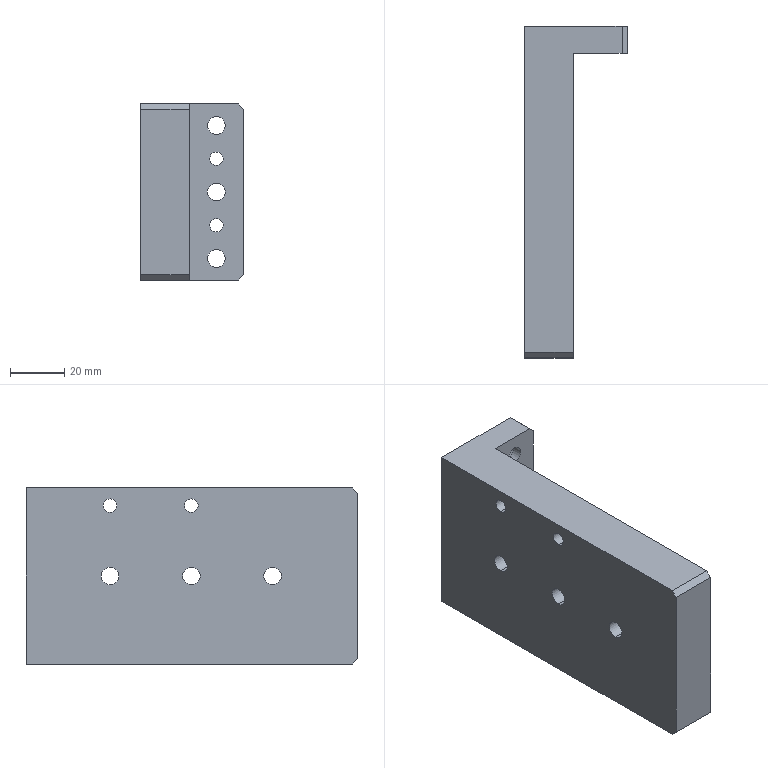Part | SolidWorks | features HoleWzd 4, Cut 2, ICE 2, MoveFace 2, Chamfer 1, Extrusion 1, LibraryFeature 1 | 1 solid | 50 faces | box 38 x 122.5 x 65 mm | volume 149829 mm3 | cylinder 32 | plane 18 | commonest cylinder face diameters 11 x12 5 x8 6.5 x6 6.6 x6
STEP:
#1=CARTESIAN_POINT('',(-8.,31.5,60.75));
#2=VERTEX_POINT('',#1);
#3=CARTESIAN_POINT('',(-8.,31.5,54.25));
#4=VERTEX_POINT('',#3);
#5=CARTESIAN_POINT('',(-8.,31.5,57.5));
#6=DIRECTION('',(1.,0.,0.));
#7=DIRECTION('',(0.,0.,-1.));
#8=AXIS2_PLACEMENT_3D('',#5,#6,#7);
#9=CIRCLE('',#8,3.25);
#10=EDGE_CURVE('',#2,#4,#9,.T.);
#11=ORIENTED_EDGE('',*,*,#10,.F.);
#12=CARTESIAN_POINT('',(3.,31.5,60.75));
#13=VERTEX_POINT('',#12);
#14=CARTESIAN_POINT('',(10.,31.5,60.75));
#15=DIRECTION('',(1.,0.,0.));
#16=VECTOR('',#15,1000.);
#17=LINE('',#14,#16);
#18=EDGE_CURVE('',#2,#13,#17,.T.);
#19=ORIENTED_EDGE('',*,*,#18,.T.);
#20=CARTESIAN_POINT('',(3.,31.5,54.25));
#21=VERTEX_POINT('',#20);
#22=CARTESIAN_POINT('',(3.,31.5,57.5));
#23=DIRECTION('',(1.,0.,0.));
#24=DIRECTION('',(0.,0.,-1.));
#25=AXIS2_PLACEMENT_3D('',#22,#23,#24);
#26=CIRCLE('',#25,3.25);
#27=EDGE_CURVE('',#13,#21,#26,.T.);
#28=ORIENTED_EDGE('',*,*,#27,.T.);
#29=CARTESIAN_POINT('',(10.,31.5,54.25));
#30=DIRECTION('',(1.,0.,0.));
#31=VECTOR('',#30,1000.);
#32=LINE('',#29,#31);
#33=EDGE_CURVE('',#4,#21,#32,.T.);
#34=ORIENTED_EDGE('',*,*,#33,.F.);
#35=EDGE_LOOP('',(#11,#19,#28,#34));
#36=FACE_OUTER_BOUND('',#35,.T.);
#37=CARTESIAN_POINT('',(10.,31.5,57.5));
#38=DIRECTION('',(1.,0.,0.));
#39=DIRECTION('',(0.,0.,-1.));
#40=AXIS2_PLACEMENT_3D('',#37,#38,#39);
#41=CYLINDRICAL_SURFACE('',#40,3.25);
#42=ADVANCED_FACE('',(#36),#41,.F.);
#43=CARTESIAN_POINT('',(3.,31.5,63.));
#44=VERTEX_POINT('',#43);
#45=CARTESIAN_POINT('',(3.,31.5,52.));
#46=VERTEX_POINT('',#45);
#47=CARTESIAN_POINT('',(3.,31.5,57.5));
#48=DIRECTION('',(1.,0.,0.));
#49=DIRECTION('',(0.,0.,-1.));
#50=AXIS2_PLACEMENT_3D('',#47,#48,#49);
#51=CIRCLE('',#50,5.5);
#52=EDGE_CURVE('',#44,#46,#51,.T.);
#53=ORIENTED_EDGE('',*,*,#52,.F.);
#54=CARTESIAN_POINT('',(10.,31.5,63.));
#55=VERTEX_POINT('',#54);
#56=CARTESIAN_POINT('',(10.,31.5,63.));
#57=DIRECTION('',(1.,0.,0.));
#58=VECTOR('',#57,1000.);
#59=LINE('',#56,#58);
#60=EDGE_CURVE('',#44,#55,#59,.T.);
#61=ORIENTED_EDGE('',*,*,#60,.T.);
#62=CARTESIAN_POINT('',(10.,31.5,52.));
#63=VERTEX_POINT('',#62);
#64=CARTESIAN_POINT('',(10.,31.5,57.5));
#65=DIRECTION('',(1.,0.,0.));
#66=DIRECTION('',(0.,0.,-1.));
#67=AXIS2_PLACEMENT_3D('',#64,#65,#66);
#68=CIRCLE('',#67,5.5);
#69=EDGE_CURVE('',#55,#63,#68,.T.);
#70=ORIENTED_EDGE('',*,*,#69,.T.);
#71=CARTESIAN_POINT('',(10.,31.5,52.));
#72=DIRECTION('',(1.,0.,0.));
#73=VECTOR('',#72,1000.);
#74=LINE('',#71,#73);
#75=EDGE_CURVE('',#46,#63,#74,.T.);
#76=ORIENTED_EDGE('',*,*,#75,.F.);
#77=EDGE_LOOP('',(#53,#61,#70,#76));
#78=FACE_OUTER_BOUND('',#77,.T.);
#79=CARTESIAN_POINT('',(10.,31.5,57.5));
#80=DIRECTION('',(1.,0.,0.));
#81=DIRECTION('',(0.,0.,-1.));
#82=AXIS2_PLACEMENT_3D('',#79,#80,#81);
#83=CYLINDRICAL_SURFACE('',#82,5.5);
#84=ADVANCED_FACE('',(#78),#83,.F.);
#85=CARTESIAN_POINT('',(-8.,61.5,60.75));
#86=VERTEX_POINT('',#85);
#87=CARTESIAN_POINT('',(-8.,61.5,54.25));
#88=VERTEX_POINT('',#87);
#89=CARTESIAN_POINT('',(-8.,61.5,57.5));
#90=DIRECTION('',(1.,0.,0.));
#91=DIRECTION('',(0.,0.,-1.));
#92=AXIS2_PLACEMENT_3D('',#89,#90,#91);
#93=CIRCLE('',#92,3.25);
#94=EDGE_CURVE('',#86,#88,#93,.T.);
#95=ORIENTED_EDGE('',*,*,#94,.F.);
#96=CARTESIAN_POINT('',(3.,61.5,60.75));
#97=VERTEX_POINT('',#96);
#98=CARTESIAN_POINT('',(10.,61.5,60.75));
#99=DIRECTION('',(1.,0.,0.));
#100=VECTOR('',#99,1000.);
#101=LINE('',#98,#100);
#102=EDGE_CURVE('',#86,#97,#101,.T.);
#103=ORIENTED_EDGE('',*,*,#102,.T.);
#104=CARTESIAN_POINT('',(3.,61.5,54.25));
#105=VERTEX_POINT('',#104);
#106=CARTESIAN_POINT('',(3.,61.5,57.5));
#107=DIRECTION('',(1.,0.,0.));
#108=DIRECTION('',(0.,0.,-1.));
#109=AXIS2_PLACEMENT_3D('',#106,#107,#108);
#110=CIRCLE('',#109,3.25);
#111=EDGE_CURVE('',#97,#105,#110,.T.);
#112=ORIENTED_EDGE('',*,*,#111,.T.);
#113=CARTESIAN_POINT('',(10.,61.5,54.25));
#114=DIRECTION('',(1.,0.,0.));
#115=VECTOR('',#114,1000.);
#116=LINE('',#113,#115);
#117=EDGE_CURVE('',#88,#105,#116,.T.);
#118=ORIENTED_EDGE('',*,*,#117,.F.);
#119=EDGE_LOOP('',(#95,#103,#112,#118));
#120=FACE_OUTER_BOUND('',#119,.T.);
#121=CARTESIAN_POINT('',(10.,61.5,57.5));
#122=DIRECTION('',(1.,0.,0.));
#123=DIRECTION('',(0.,0.,-1.));
#124=AXIS2_PLACEMENT_3D('',#121,#122,#123);
#125=CYLINDRICAL_SURFACE('',#124,3.25);
#126=ADVANCED_FACE('',(#120),#125,.F.);
#127=CARTESIAN_POINT('',(3.,61.5,63.));
#128=VERTEX_POINT('',#127);
#129=CARTESIAN_POINT('',(3.,61.5,52.));
#130=VERTEX_POINT('',#129);
#131=CARTESIAN_POINT('',(3.,61.5,57.5));
#132=DIRECTION('',(1.,0.,0.));
#133=DIRECTION('',(0.,0.,-1.));
#134=AXIS2_PLACEMENT_3D('',#131,#132,#133);
#135=CIRCLE('',#134,5.5);
#136=EDGE_CURVE('',#128,#130,#135,.T.);
#137=ORIENTED_EDGE('',*,*,#136,.F.);
#138=CARTESIAN_POINT('',(10.,61.5,63.));
#139=VERTEX_POINT('',#138);
#140=CARTESIAN_POINT('',(10.,61.5,63.));
#141=DIRECTION('',(1.,0.,0.));
#142=VECTOR('',#141,1000.);
#143=LINE('',#140,#142);
#144=EDGE_CURVE('',#128,#139,#143,.T.);
#145=ORIENTED_EDGE('',*,*,#144,.T.);
#146=CARTESIAN_POINT('',(10.,61.5,52.));
#147=VERTEX_POINT('',#146);
#148=CARTESIAN_POINT('',(10.,61.5,57.5));
#149=DIRECTION('',(1.,0.,0.));
#150=DIRECTION('',(0.,0.,-1.));
#151=AXIS2_PLACEMENT_3D('',#148,#149,#150);
#152=CIRCLE('',#151,5.5);
#153=EDGE_CURVE('',#139,#147,#152,.T.);
#154=ORIENTED_EDGE('',*,*,#153,.T.);
#155=CARTESIAN_POINT('',(10.,61.5,52.));
#156=DIRECTION('',(1.,0.,0.));
#157=VECTOR('',#156,1000.);
#158=LINE('',#155,#157);
#159=EDGE_CURVE('',#130,#147,#158,.T.);
#160=ORIENTED_EDGE('',*,*,#159,.F.);
#161=EDGE_LOOP('',(#137,#145,#154,#160));
#162=FACE_OUTER_BOUND('',#161,.T.);
#163=CARTESIAN_POINT('',(10.,61.5,57.5));
#164=DIRECTION('',(1.,0.,0.));
#165=DIRECTION('',(0.,0.,-1.));
#166=AXIS2_PLACEMENT_3D('',#163,#164,#165);
#167=CYLINDRICAL_SURFACE('',#166,5.5);
#168=ADVANCED_FACE('',(#162),#167,.F.);
#169=CARTESIAN_POINT('',(-8.,91.5,60.75));
#170=VERTEX_POINT('',#169);
#171=CARTESIAN_POINT('',(-8.,91.5,54.25));
#172=VERTEX_POINT('',#171);
#173=CARTESIAN_POINT('',(-8.,91.5,57.5));
#174=DIRECTION('',(1.,0.,0.));
#175=DIRECTION('',(0.,0.,-1.));
#176=AXIS2_PLACEMENT_3D('',#173,#174,#175);
#177=CIRCLE('',#176,3.25);
#178=EDGE_CURVE('',#170,#172,#177,.T.);
#179=ORIENTED_EDGE('',*,*,#178,.F.);
#180=CARTESIAN_POINT('',(3.,91.5,60.75));
#181=VERTEX_POINT('',#180);
#182=CARTESIAN_POINT('',(10.,91.5,60.75));
#183=DIRECTION('',(1.,0.,0.));
#184=VECTOR('',#183,1000.);
#185=LINE('',#182,#184);
#186=EDGE_CURVE('',#170,#181,#185,.T.);
#187=ORIENTED_EDGE('',*,*,#186,.T.);
#188=CARTESIAN_POINT('',(3.,91.5,54.25));
#189=VERTEX_POINT('',#188);
#190=CARTESIAN_POINT('',(3.,91.5,57.5));
#191=DIRECTION('',(1.,0.,0.));
#192=DIRECTION('',(0.,0.,-1.));
#193=AXIS2_PLACEMENT_3D('',#190,#191,#192);
#194=CIRCLE('',#193,3.25);
#195=EDGE_CURVE('',#181,#189,#194,.T.);
#196=ORIENTED_EDGE('',*,*,#195,.T.);
#197=CARTESIAN_POINT('',(10.,91.5,54.25));
#198=DIRECTION('',(1.,0.,0.));
#199=VECTOR('',#198,1000.);
#200=LINE('',#197,#199);
#201=EDGE_CURVE('',#172,#189,#200,.T.);
#202=ORIENTED_EDGE('',*,*,#201,.F.);
#203=EDGE_LOOP('',(#179,#187,#196,#202));
#204=FACE_OUTER_BOUND('',#203,.T.);
#205=CARTESIAN_POINT('',(10.,91.5,57.5));
#206=DIRECTION('',(1.,0.,0.));
#207=DIRECTION('',(0.,0.,-1.));
#208=AXIS2_PLACEMENT_3D('',#205,#206,#207);
#209=CYLINDRICAL_SURFACE('',#208,3.25);
#210=ADVANCED_FACE('',(#204),#209,.F.);
#211=CARTESIAN_POINT('',(3.,91.5,63.));
#212=VERTEX_POINT('',#211);
#213=CARTESIAN_POINT('',(3.,91.5,52.));
#214=VERTEX_POINT('',#213);
#215=CARTESIAN_POINT('',(3.,91.5,57.5));
#216=DIRECTION('',(1.,0.,0.));
#217=DIRECTION('',(0.,0.,-1.));
#218=AXIS2_PLACEMENT_3D('',#215,#216,#217);
#219=CIRCLE('',#218,5.5);
#220=EDGE_CURVE('',#212,#214,#219,.T.);
#221=ORIENTED_EDGE('',*,*,#220,.F.);
#222=CARTESIAN_POINT('',(10.,91.5,63.));
#223=VERTEX_POINT('',#222);
#224=CARTESIAN_POINT('',(10.,91.5,63.));
#225=DIRECTION('',(1.,0.,0.));
#226=VECTOR('',#225,1000.);
#227=LINE('',#224,#226);
#228=EDGE_CURVE('',#212,#223,#227,.T.);
#229=ORIENTED_EDGE('',*,*,#228,.T.);
#230=CARTESIAN_POINT('',(10.,91.5,52.));
#231=VERTEX_POINT('',#230);
#232=CARTESIAN_POINT('',(10.,91.5,57.5));
#233=DIRECTION('',(1.,0.,0.));
#234=DIRECTION('',(0.,0.,-1.));
#235=AXIS2_PLACEMENT_3D('',#232,#233,#234);
#236=CIRCLE('',#235,5.5);
#237=EDGE_CURVE('',#223,#231,#236,.T.);
#238=ORIENTED_EDGE('',*,*,#237,.T.);
#239=CARTESIAN_POINT('',(10.,91.5,52.));
#240=DIRECTION('',(1.,0.,0.));
#241=VECTOR('',#240,1000.);
#242=LINE('',#239,#241);
#243=EDGE_CURVE('',#214,#231,#242,.T.);
#244=ORIENTED_EDGE('',*,*,#243,.F.);
#245=EDGE_LOOP('',(#221,#229,#238,#244));
#246=FACE_OUTER_BOUND('',#245,.T.);
#247=CARTESIAN_POINT('',(10.,91.5,57.5));
#248=DIRECTION('',(1.,0.,0.));
#249=DIRECTION('',(0.,0.,-1.));
#250=AXIS2_PLACEMENT_3D('',#247,#248,#249);
#251=CYLINDRICAL_SURFACE('',#250,5.5);
#252=ADVANCED_FACE('',(#246),#251,.F.);
#253=CARTESIAN_POINT('',(-8.,91.5,86.));
#254=VERTEX_POINT('',#253);
#255=CARTESIAN_POINT('',(-8.,91.5,81.));
#256=VERTEX_POINT('',#255);
#257=CARTESIAN_POINT('',(-8.,91.5,83.5));
#258=DIRECTION('',(1.,0.,0.));
#259=DIRECTION('',(0.,0.,-1.));
#260=AXIS2_PLACEMENT_3D('',#257,#258,#259);
#261=CIRCLE('',#260,2.5);
#262=EDGE_CURVE('',#254,#256,#261,.T.);
#263=ORIENTED_EDGE('',*,*,#262,.F.);
#264=CARTESIAN_POINT('',(10.,91.5,86.));
#265=VERTEX_POINT('',#264);
#266=CARTESIAN_POINT('',(10.,91.5,86.));
#267=DIRECTION('',(1.,0.,0.));
#268=VECTOR('',#267,1000.);
#269=LINE('',#266,#268);
#270=EDGE_CURVE('',#254,#265,#269,.T.);
#271=ORIENTED_EDGE('',*,*,#270,.T.);
#272=CARTESIAN_POINT('',(10.,91.5,81.));
#273=VERTEX_POINT('',#272);
#274=CARTESIAN_POINT('',(10.,91.5,83.5));
#275=DIRECTION('',(1.,0.,0.));
#276=DIRECTION('',(0.,0.,-1.));
#277=AXIS2_PLACEMENT_3D('',#274,#275,#276);
#278=CIRCLE('',#277,2.5);
#279=EDGE_CURVE('',#265,#273,#278,.T.);
#280=ORIENTED_EDGE('',*,*,#279,.T.);
#281=CARTESIAN_POINT('',(10.,91.5,81.));
#282=DIRECTION('',(1.,0.,0.));
#283=VECTOR('',#282,1000.);
#284=LINE('',#281,#283);
#285=EDGE_CURVE('',#256,#273,#284,.T.);
#286=ORIENTED_EDGE('',*,*,#285,.F.);
#287=EDGE_LOOP('',(#263,#271,#280,#286));
#288=FACE_OUTER_BOUND('',#287,.T.);
#289=CARTESIAN_POINT('',(10.,91.5,83.5));
#290=DIRECTION('',(1.,0.,0.));
#291=DIRECTION('',(0.,0.,-1.));
#292=AXIS2_PLACEMENT_3D('',#289,#290,#291);
#293=CYLINDRICAL_SURFACE('',#292,2.5);
#294=ADVANCED_FACE('',(#288),#293,.F.);
#295=CARTESIAN_POINT('',(-8.,61.5,86.));
#296=VERTEX_POINT('',#295);
#297=CARTESIAN_POINT('',(-8.,61.5,81.));
#298=VERTEX_POINT('',#297);
#299=CARTESIAN_POINT('',(-8.,61.5,83.5));
#300=DIRECTION('',(1.,0.,0.));
#301=DIRECTION('',(0.,0.,-1.));
#302=AXIS2_PLACEMENT_3D('',#299,#300,#301);
#303=CIRCLE('',#302,2.5);
#304=EDGE_CURVE('',#296,#298,#303,.T.);
#305=ORIENTED_EDGE('',*,*,#304,.F.);
#306=CARTESIAN_POINT('',(10.,61.5,86.));
#307=VERTEX_POINT('',#306);
#308=CARTESIAN_POINT('',(10.,61.5,86.));
#309=DIRECTION('',(1.,0.,0.));
#310=VECTOR('',#309,1000.);
#311=LINE('',#308,#310);
#312=EDGE_CURVE('',#296,#307,#311,.T.);
#313=ORIENTED_EDGE('',*,*,#312,.T.);
#314=CARTESIAN_POINT('',(10.,61.5,81.));
#315=VERTEX_POINT('',#314);
#316=CARTESIAN_POINT('',(10.,61.5,83.5));
#317=DIRECTION('',(1.,0.,0.));
#318=DIRECTION('',(0.,0.,-1.));
#319=AXIS2_PLACEMENT_3D('',#316,#317,#318);
#320=CIRCLE('',#319,2.5);
#321=EDGE_CURVE('',#307,#315,#320,.T.);
#322=ORIENTED_EDGE('',*,*,#321,.T.);
#323=CARTESIAN_POINT('',(10.,61.5,81.));
#324=DIRECTION('',(1.,0.,0.));
#325=VECTOR('',#324,1000.);
#326=LINE('',#323,#325);
#327=EDGE_CURVE('',#298,#315,#326,.T.);
#328=ORIENTED_EDGE('',*,*,#327,.F.);
#329=EDGE_LOOP('',(#305,#313,#322,#328));
#330=FACE_OUTER_BOUND('',#329,.T.);
#331=CARTESIAN_POINT('',(10.,61.5,83.5));
#332=DIRECTION('',(1.,0.,0.));
#333=DIRECTION('',(0.,0.,-1.));
#334=AXIS2_PLACEMENT_3D('',#331,#332,#333);
#335=CYLINDRICAL_SURFACE('',#334,2.5);
#336=ADVANCED_FACE('',(#330),#335,.F.);
#337=CARTESIAN_POINT('',(20.,112.5,42.75));
#338=VERTEX_POINT('',#337);
#339=CARTESIAN_POINT('',(20.,112.5,47.75));
#340=VERTEX_POINT('',#339);
#341=CARTESIAN_POINT('',(20.,112.5,45.25));
#342=DIRECTION('',(0.,1.,0.));
#343=DIRECTION('',(-1.,0.,0.));
#344=AXIS2_PLACEMENT_3D('',#341,#342,#343);
#345=CIRCLE('',#344,2.5);
#346=EDGE_CURVE('',#338,#340,#345,.T.);
#347=ORIENTED_EDGE('',*,*,#346,.F.);
#348=CARTESIAN_POINT('',(20.,122.5,42.75));
#349=VERTEX_POINT('',#348);
#350=CARTESIAN_POINT('',(20.,122.5,42.75));
#351=DIRECTION('',(0.,1.,0.));
#352=VECTOR('',#351,1000.);
#353=LINE('',#350,#352);
#354=EDGE_CURVE('',#338,#349,#353,.T.);
#355=ORIENTED_EDGE('',*,*,#354,.T.);
#356=CARTESIAN_POINT('',(20.,122.5,47.75));
#357=VERTEX_POINT('',#356);
#358=CARTESIAN_POINT('',(20.,122.5,45.25));
#359=DIRECTION('',(0.,1.,0.));
#360=DIRECTION('',(0.,0.,1.));
#361=AXIS2_PLACEMENT_3D('',#358,#359,#360);
#362=CIRCLE('',#361,2.5);
#363=EDGE_CURVE('',#349,#357,#362,.T.);
#364=ORIENTED_EDGE('',*,*,#363,.T.);
#365=CARTESIAN_POINT('',(20.,122.5,47.75));
#366=DIRECTION('',(0.,1.,0.));
#367=VECTOR('',#366,1000.);
#368=LINE('',#365,#367);
#369=EDGE_CURVE('',#340,#357,#368,.T.);
#370=ORIENTED_EDGE('',*,*,#369,.F.);
#371=EDGE_LOOP('',(#347,#355,#364,#370));
#372=FACE_OUTER_BOUND('',#371,.T.);
#373=CARTESIAN_POINT('',(20.,122.5,45.25));
#374=DIRECTION('',(0.,1.,0.));
#375=DIRECTION('',(0.,0.,1.));
#376=AXIS2_PLACEMENT_3D('',#373,#374,#375);
#377=CYLINDRICAL_SURFACE('',#376,2.5);
#378=ADVANCED_FACE('',(#372),#377,.F.);
#379=CARTESIAN_POINT('',(20.,112.5,67.25));
#380=VERTEX_POINT('',#379);
#381=CARTESIAN_POINT('',(20.,112.5,72.25));
#382=VERTEX_POINT('',#381);
#383=CARTESIAN_POINT('',(20.,112.5,69.75));
#384=DIRECTION('',(0.,1.,0.));
#385=DIRECTION('',(-1.,0.,0.));
#386=AXIS2_PLACEMENT_3D('',#383,#384,#385);
#387=CIRCLE('',#386,2.5);
#388=EDGE_CURVE('',#380,#382,#387,.T.);
#389=ORIENTED_EDGE('',*,*,#388,.F.);
#390=CARTESIAN_POINT('',(20.,122.5,67.25));
#391=VERTEX_POINT('',#390);
#392=CARTESIAN_POINT('',(20.,122.5,67.25));
#393=DIRECTION('',(0.,1.,0.));
#394=VECTOR('',#393,1000.);
#395=LINE('',#392,#394);
#396=EDGE_CURVE('',#380,#391,#395,.T.);
#397=ORIENTED_EDGE('',*,*,#396,.T.);
#398=CARTESIAN_POINT('',(20.,122.5,72.25));
#399=VERTEX_POINT('',#398);
#400=CARTESIAN_POINT('',(20.,122.5,69.75));
#401=DIRECTION('',(0.,1.,0.));
#402=DIRECTION('',(0.,0.,1.));
#403=AXIS2_PLACEMENT_3D('',#400,#401,#402);
#404=CIRCLE('',#403,2.5);
#405=EDGE_CURVE('',#391,#399,#404,.T.);
#406=ORIENTED_EDGE('',*,*,#405,.T.);
#407=CARTESIAN_POINT('',(20.,122.5,72.25));
#408=DIRECTION('',(0.,1.,0.));
#409=VECTOR('',#408,1000.);
#410=LINE('',#407,#409);
#411=EDGE_CURVE('',#382,#399,#410,.T.);
#412=ORIENTED_EDGE('',*,*,#411,.F.);
#413=EDGE_LOOP('',(#389,#397,#406,#412));
#414=FACE_OUTER_BOUND('',#413,.T.);
#415=CARTESIAN_POINT('',(20.,122.5,69.75));
#416=DIRECTION('',(0.,1.,0.));
#417=DIRECTION('',(0.,0.,1.));
#418=AXIS2_PLACEMENT_3D('',#415,#416,#417);
#419=CYLINDRICAL_SURFACE('',#418,2.5);
#420=ADVANCED_FACE('',(#414),#419,.F.);
#421=CARTESIAN_POINT('',(20.,116.1,76.5));
#422=VERTEX_POINT('',#421);
#423=CARTESIAN_POINT('',(20.,116.1,87.5));
#424=VERTEX_POINT('',#423);
#425=CARTESIAN_POINT('',(20.,116.1,82.));
#426=DIRECTION('',(0.,1.,0.));
#427=DIRECTION('',(0.,0.,1.));
#428=AXIS2_PLACEMENT_3D('',#425,#426,#427);
#429=CIRCLE('',#428,5.5);
#430=EDGE_CURVE('',#422,#424,#429,.T.);
#431=ORIENTED_EDGE('',*,*,#430,.F.);
#432=CARTESIAN_POINT('',(20.,122.5,76.5));
#433=VERTEX_POINT('',#432);
#434=CARTESIAN_POINT('',(20.,122.5,76.5));
#435=DIRECTION('',(0.,1.,0.));
#436=VECTOR('',#435,1000.);
#437=LINE('',#434,#436);
#438=EDGE_CURVE('',#422,#433,#437,.T.);
#439=ORIENTED_EDGE('',*,*,#438,.T.);
#440=CARTESIAN_POINT('',(20.,122.5,87.5));
#441=VERTEX_POINT('',#440);
#442=CARTESIAN_POINT('',(20.,122.5,82.));
#443=DIRECTION('',(0.,1.,0.));
#444=DIRECTION('',(0.,0.,1.));
#445=AXIS2_PLACEMENT_3D('',#442,#443,#444);
#446=CIRCLE('',#445,5.5);
#447=EDGE_CURVE('',#433,#441,#446,.T.);
#448=ORIENTED_EDGE('',*,*,#447,.T.);
#449=CARTESIAN_POINT('',(20.,122.5,87.5));
#450=DIRECTION('',(0.,1.,0.));
#451=VECTOR('',#450,1000.);
#452=LINE('',#449,#451);
#453=EDGE_CURVE('',#424,#441,#452,.T.);
#454=ORIENTED_EDGE('',*,*,#453,.F.);
#455=EDGE_LOOP('',(#431,#439,#448,#454));
#456=FACE_OUTER_BOUND('',#455,.T.);
#457=CARTESIAN_POINT('',(20.,122.5,82.));
#458=DIRECTION('',(0.,1.,0.));
#459=DIRECTION('',(0.,0.,1.));
#460=AXIS2_PLACEMENT_3D('',#457,#458,#459);
#461=CYLINDRICAL_SURFACE('',#460,5.5);
#462=ADVANCED_FACE('',(#456),#461,.F.);
#463=CARTESIAN_POINT('',(20.,112.5,78.7));
#464=VERTEX_POINT('',#463);
#465=CARTESIAN_POINT('',(20.,112.5,85.3));
#466=VERTEX_POINT('',#465);
#467=CARTESIAN_POINT('',(20.,112.5,82.));
#468=DIRECTION('',(0.,1.,0.));
#469=DIRECTION('',(-1.,0.,0.));
#470=AXIS2_PLACEMENT_3D('',#467,#468,#469);
#471=CIRCLE('',#470,3.3);
#472=EDGE_CURVE('',#464,#466,#471,.T.);
#473=ORIENTED_EDGE('',*,*,#472,.F.);
#474=CARTESIAN_POINT('',(20.,116.1,78.7));
#475=VERTEX_POINT('',#474);
#476=CARTESIAN_POINT('',(20.,122.5,78.7));
#477=DIRECTION('',(0.,1.,0.));
#478=VECTOR('',#477,1000.);
#479=LINE('',#476,#478);
#480=EDGE_CURVE('',#464,#475,#479,.T.);
#481=ORIENTED_EDGE('',*,*,#480,.T.);
#482=CARTESIAN_POINT('',(20.,116.1,85.3));
#483=VERTEX_POINT('',#482);
#484=CARTESIAN_POINT('',(20.,116.1,82.));
#485=DIRECTION('',(0.,1.,0.));
#486=DIRECTION('',(0.,0.,1.));
#487=AXIS2_PLACEMENT_3D('',#484,#485,#486);
#488=CIRCLE('',#487,3.3);
#489=EDGE_CURVE('',#475,#483,#488,.T.);
#490=ORIENTED_EDGE('',*,*,#489,.T.);
#491=CARTESIAN_POINT('',(20.,122.5,85.3));
#492=DIRECTION('',(0.,1.,0.));
#493=VECTOR('',#492,1000.);
#494=LINE('',#491,#493);
#495=EDGE_CURVE('',#466,#483,#494,.T.);
#496=ORIENTED_EDGE('',*,*,#495,.F.);
#497=EDGE_LOOP('',(#473,#481,#490,#496));
#498=FACE_OUTER_BOUND('',#497,.T.);
#499=CARTESIAN_POINT('',(20.,122.5,82.));
#500=DIRECTION('',(0.,1.,0.));
#501=DIRECTION('',(0.,0.,1.));
#502=AXIS2_PLACEMENT_3D('',#499,#500,#501);
#503=CYLINDRICAL_SURFACE('',#502,3.3);
#504=ADVANCED_FACE('',(#498),#503,.F.);
#505=CARTESIAN_POINT('',(20.,116.1,27.5));
#506=VERTEX_POINT('',#505);
#507=CARTESIAN_POINT('',(20.,116.1,38.5));
#508=VERTEX_POINT('',#507);
#509=CARTESIAN_POINT('',(20.,116.1,33.));
#510=DIRECTION('',(0.,1.,0.));
#511=DIRECTION('',(0.,0.,1.));
#512=AXIS2_PLACEMENT_3D('',#509,#510,#511);
#513=CIRCLE('',#512,5.5);
#514=EDGE_CURVE('',#506,#508,#513,.T.);
#515=ORIENTED_EDGE('',*,*,#514,.F.);
#516=CARTESIAN_POINT('',(20.,122.5,27.5));
#517=VERTEX_POINT('',#516);
#518=CARTESIAN_POINT('',(20.,122.5,27.5));
#519=DIRECTION('',(0.,1.,0.));
#520=VECTOR('',#519,1000.);
#521=LINE('',#518,#520);
#522=EDGE_CURVE('',#506,#517,#521,.T.);
#523=ORIENTED_EDGE('',*,*,#522,.T.);
#524=CARTESIAN_POINT('',(20.,122.5,38.5));
#525=VERTEX_POINT('',#524);
#526=CARTESIAN_POINT('',(20.,122.5,33.));
#527=DIRECTION('',(0.,1.,0.));
#528=DIRECTION('',(0.,0.,1.));
#529=AXIS2_PLACEMENT_3D('',#526,#527,#528);
#530=CIRCLE('',#529,5.5);
#531=EDGE_CURVE('',#517,#525,#530,.T.);
#532=ORIENTED_EDGE('',*,*,#531,.T.);
#533=CARTESIAN_POINT('',(20.,122.5,38.5));
#534=DIRECTION('',(0.,1.,0.));
#535=VECTOR('',#534,1000.);
#536=LINE('',#533,#535);
#537=EDGE_CURVE('',#508,#525,#536,.T.);
#538=ORIENTED_EDGE('',*,*,#537,.F.);
#539=EDGE_LOOP('',(#515,#523,#532,#538));
#540=FACE_OUTER_BOUND('',#539,.T.);
#541=CARTESIAN_POINT('',(20.,122.5,33.));
#542=DIRECTION('',(0.,1.,0.));
#543=DIRECTION('',(0.,0.,1.));
#544=AXIS2_PLACEMENT_3D('',#541,#542,#543);
#545=CYLINDRICAL_SURFACE('',#544,5.5);
#546=ADVANCED_FACE('',(#540),#545,.F.);
#547=CARTESIAN_POINT('',(20.,112.5,29.7));
#548=VERTEX_POINT('',#547);
#549=CARTESIAN_POINT('',(20.,112.5,36.3));
#550=VERTEX_POINT('',#549);
#551=CARTESIAN_POINT('',(20.,112.5,33.));
#552=DIRECTION('',(0.,1.,0.));
#553=DIRECTION('',(-1.,0.,0.));
#554=AXIS2_PLACEMENT_3D('',#551,#552,#553);
#555=CIRCLE('',#554,3.3);
#556=EDGE_CURVE('',#548,#550,#555,.T.);
#557=ORIENTED_EDGE('',*,*,#556,.F.);
#558=CARTESIAN_POINT('',(20.,116.1,29.7));
#559=VERTEX_POINT('',#558);
#560=CARTESIAN_POINT('',(20.,122.5,29.7));
#561=DIRECTION('',(0.,1.,0.));
#562=VECTOR('',#561,1000.);
#563=LINE('',#560,#562);
#564=EDGE_CURVE('',#548,#559,#563,.T.);
#565=ORIENTED_EDGE('',*,*,#564,.T.);
#566=CARTESIAN_POINT('',(20.,116.1,36.3));
#567=VERTEX_POINT('',#566);
#568=CARTESIAN_POINT('',(20.,116.1,33.));
#569=DIRECTION('',(0.,1.,0.));
#570=DIRECTION('',(0.,0.,1.));
#571=AXIS2_PLACEMENT_3D('',#568,#569,#570);
#572=CIRCLE('',#571,3.3);
#573=EDGE_CURVE('',#559,#567,#572,.T.);
#574=ORIENTED_EDGE('',*,*,#573,.T.);
#575=CARTESIAN_POINT('',(20.,122.5,36.3));
#576=DIRECTION('',(0.,1.,0.));
#577=VECTOR('',#576,1000.);
#578=LINE('',#575,#577);
#579=EDGE_CURVE('',#550,#567,#578,.T.);
#580=ORIENTED_EDGE('',*,*,#579,.F.);
#581=EDGE_LOOP('',(#557,#565,#574,#580));
#582=FACE_OUTER_BOUND('',#581,.T.);
#583=CARTESIAN_POINT('',(20.,122.5,33.));
#584=DIRECTION('',(0.,1.,0.));
#585=DIRECTION('',(0.,0.,1.));
#586=AXIS2_PLACEMENT_3D('',#583,#584,#585);
#587=CYLINDRICAL_SURFACE('',#586,3.3);
#588=ADVANCED_FACE('',(#582),#587,.F.);
#589=CARTESIAN_POINT('',(20.,116.1,52.));
#590=VERTEX_POINT('',#589);
#591=CARTESIAN_POINT('',(20.,116.1,63.));
#592=VERTEX_POINT('',#591);
#593=CARTESIAN_POINT('',(20.,116.1,57.5));
#594=DIRECTION('',(0.,1.,0.));
#595=DIRECTION('',(0.,0.,1.));
#596=AXIS2_PLACEMENT_3D('',#593,#594,#595);
#597=CIRCLE('',#596,5.5);
#598=EDGE_CURVE('',#590,#592,#597,.T.);
#599=ORIENTED_EDGE('',*,*,#598,.F.);
#600=CARTESIAN_POINT('',(20.,122.5,52.));
#601=VERTEX_POINT('',#600);
#602=CARTESIAN_POINT('',(20.,122.5,52.));
#603=DIRECTION('',(0.,1.,0.));
#604=VECTOR('',#603,1000.);
#605=LINE('',#602,#604);
#606=EDGE_CURVE('',#590,#601,#605,.T.);
#607=ORIENTED_EDGE('',*,*,#606,.T.);
#608=CARTESIAN_POINT('',(20.,122.5,63.));
#609=VERTEX_POINT('',#608);
#610=CARTESIAN_POINT('',(20.,122.5,57.5));
#611=DIRECTION('',(0.,1.,0.));
#612=DIRECTION('',(0.,0.,1.));
#613=AXIS2_PLACEMENT_3D('',#610,#611,#612);
#614=CIRCLE('',#613,5.5);
#615=EDGE_CURVE('',#601,#609,#614,.T.);
#616=ORIENTED_EDGE('',*,*,#615,.T.);
#617=CARTESIAN_POINT('',(20.,122.5,63.));
#618=DIRECTION('',(0.,1.,0.));
#619=VECTOR('',#618,1000.);
#620=LINE('',#617,#619);
#621=EDGE_CURVE('',#592,#609,#620,.T.);
#622=ORIENTED_EDGE('',*,*,#621,.F.);
#623=EDGE_LOOP('',(#599,#607,#616,#622));
#624=FACE_OUTER_BOUND('',#623,.T.);
#625=CARTESIAN_POINT('',(20.,122.5,57.5));
#626=DIRECTION('',(0.,1.,0.));
#627=DIRECTION('',(0.,0.,1.));
#628=AXIS2_PLACEMENT_3D('',#625,#626,#627);
#629=CYLINDRICAL_SURFACE('',#628,5.5);
#630=ADVANCED_FACE('',(#624),#629,.F.);
#631=CARTESIAN_POINT('',(20.,112.5,54.2));
#632=VERTEX_POINT('',#631);
#633=CARTESIAN_POINT('',(20.,112.5,60.8));
#634=VERTEX_POINT('',#633);
#635=CARTESIAN_POINT('',(20.,112.5,57.5));
#636=DIRECTION('',(0.,1.,0.));
#637=DIRECTION('',(-1.,0.,0.));
#638=AXIS2_PLACEMENT_3D('',#635,#636,#637);
#639=CIRCLE('',#638,3.3);
#640=EDGE_CURVE('',#632,#634,#639,.T.);
#641=ORIENTED_EDGE('',*,*,#640,.F.);
#642=CARTESIAN_POINT('',(20.,116.1,54.2));
#643=VERTEX_POINT('',#642);
#644=CARTESIAN_POINT('',(20.,122.5,54.2));
#645=DIRECTION('',(0.,1.,0.));
#646=VECTOR('',#645,1000.);
#647=LINE('',#644,#646);
#648=EDGE_CURVE('',#632,#643,#647,.T.);
#649=ORIENTED_EDGE('',*,*,#648,.T.);
#650=CARTESIAN_POINT('',(20.,116.1,60.8));
#651=VERTEX_POINT('',#650);
#652=CARTESIAN_POINT('',(20.,116.1,57.5));
#653=DIRECTION('',(0.,1.,0.));
#654=DIRECTION('',(0.,0.,1.));
#655=AXIS2_PLACEMENT_3D('',#652,#653,#654);
#656=CIRCLE('',#655,3.3);
#657=EDGE_CURVE('',#643,#651,#656,.T.);
#658=ORIENTED_EDGE('',*,*,#657,.T.);
#659=CARTESIAN_POINT('',(20.,122.5,60.8));
#660=DIRECTION('',(0.,1.,0.));
#661=VECTOR('',#660,1000.);
#662=LINE('',#659,#661);
#663=EDGE_CURVE('',#634,#651,#662,.T.);
#664=ORIENTED_EDGE('',*,*,#663,.F.);
#665=EDGE_LOOP('',(#641,#649,#658,#664));
#666=FACE_OUTER_BOUND('',#665,.T.);
#667=CARTESIAN_POINT('',(20.,122.5,57.5));
#668=DIRECTION('',(0.,1.,0.));
#669=DIRECTION('',(0.,0.,1.));
#670=AXIS2_PLACEMENT_3D('',#667,#668,#669);
#671=CYLINDRICAL_SURFACE('',#670,3.3);
#672=ADVANCED_FACE('',(#666),#671,.F.);
#673=CARTESIAN_POINT('',(10.,31.5,57.5));
#674=DIRECTION('',(1.,0.,0.));
#675=DIRECTION('',(0.,0.,-1.));
#676=AXIS2_PLACEMENT_3D('',#673,#674,#675);
#677=CIRCLE('',#676,5.5);
#678=EDGE_CURVE('',#63,#55,#677,.T.);
#679=ORIENTED_EDGE('',*,*,#678,.F.);
#680=ORIENTED_EDGE('',*,*,#69,.F.);
#681=EDGE_LOOP('',(#679,#680));
#682=FACE_BOUND('',#681,.T.);
#683=CARTESIAN_POINT('',(10.,61.5,57.5));
#684=DIRECTION('',(1.,0.,0.));
#685=DIRECTION('',(0.,0.,-1.));
#686=AXIS2_PLACEMENT_3D('',#683,#684,#685);
#687=CIRCLE('',#686,5.5);
#688=EDGE_CURVE('',#147,#139,#687,.T.);
#689=ORIENTED_EDGE('',*,*,#688,.F.);
#690=ORIENTED_EDGE('',*,*,#153,.F.);
#691=EDGE_LOOP('',(#689,#690));
#692=FACE_BOUND('',#691,.T.);
#693=CARTESIAN_POINT('',(10.,91.5,57.5));
#694=DIRECTION('',(1.,0.,0.));
#695=DIRECTION('',(0.,0.,-1.));
#696=AXIS2_PLACEMENT_3D('',#693,#694,#695);
#697=CIRCLE('',#696,5.5);
#698=EDGE_CURVE('',#231,#223,#697,.T.);
#699=ORIENTED_EDGE('',*,*,#698,.F.);
#700=ORIENTED_EDGE('',*,*,#237,.F.);
#701=EDGE_LOOP('',(#699,#700));
#702=FACE_BOUND('',#701,.T.);
#703=CARTESIAN_POINT('',(10.,91.5,83.5));
#704=DIRECTION('',(1.,0.,0.));
#705=DIRECTION('',(0.,0.,-1.));
#706=AXIS2_PLACEMENT_3D('',#703,#704,#705);
#707=CIRCLE('',#706,2.5);
#708=EDGE_CURVE('',#273,#265,#707,.T.);
#709=ORIENTED_EDGE('',*,*,#708,.F.);
#710=ORIENTED_EDGE('',*,*,#279,.F.);
#711=EDGE_LOOP('',(#709,#710));
#712=FACE_BOUND('',#711,.T.);
#713=CARTESIAN_POINT('',(10.,2.,90.));
#714=VERTEX_POINT('',#713);
#715=CARTESIAN_POINT('',(10.,112.5,90.));
#716=VERTEX_POINT('',#715);
#717=CARTESIAN_POINT('',(10.,0.,90.));
#718=DIRECTION('',(0.,1.,0.));
#719=VECTOR('',#718,1000.);
#720=LINE('',#717,#719);
#721=EDGE_CURVE('',#714,#716,#720,.T.);
#722=ORIENTED_EDGE('',*,*,#721,.F.);
#723=CARTESIAN_POINT('',(10.,0.,88.));
#724=VERTEX_POINT('',#723);
#725=CARTESIAN_POINT('',(10.,2.,90.));
#726=DIRECTION('',(0.,-0.7071,-0.7071));
#727=VECTOR('',#726,1000.);
#728=LINE('',#725,#727);
#729=EDGE_CURVE('',#714,#724,#728,.T.);
#730=ORIENTED_EDGE('',*,*,#729,.T.);
#731=CARTESIAN_POINT('',(10.,0.,27.));
#732=VERTEX_POINT('',#731);
#733=CARTESIAN_POINT('',(10.,0.,90.));
#734=DIRECTION('',(0.,0.,-1.));
#735=VECTOR('',#734,1000.);
#736=LINE('',#733,#735);
#737=EDGE_CURVE('',#724,#732,#736,.T.);
#738=ORIENTED_EDGE('',*,*,#737,.T.);
#739=CARTESIAN_POINT('',(10.,2.,25.));
#740=VERTEX_POINT('',#739);
#741=CARTESIAN_POINT('',(10.,0.,27.));
#742=DIRECTION('',(0.,0.7071,-0.7071));
#743=VECTOR('',#742,1000.);
#744=LINE('',#741,#743);
#745=EDGE_CURVE('',#732,#740,#744,.T.);
#746=ORIENTED_EDGE('',*,*,#745,.T.);
#747=CARTESIAN_POINT('',(10.,112.5,25.));
#748=VERTEX_POINT('',#747);
#749=CARTESIAN_POINT('',(10.,0.,25.));
#750=DIRECTION('',(0.,1.,0.));
#751=VECTOR('',#750,1000.);
#752=LINE('',#749,#751);
#753=EDGE_CURVE('',#740,#748,#752,.T.);
#754=ORIENTED_EDGE('',*,*,#753,.T.);
#755=CARTESIAN_POINT('',(10.,112.5,90.));
#756=DIRECTION('',(0.,0.,-1.));
#757=VECTOR('',#756,1000.);
#758=LINE('',#755,#757);
#759=EDGE_CURVE('',#716,#748,#758,.T.);
#760=ORIENTED_EDGE('',*,*,#759,.F.);
#761=EDGE_LOOP('',(#722,#730,#738,#746,#754,#760));
#762=FACE_OUTER_BOUND('',#761,.T.);
#763=CARTESIAN_POINT('',(10.,61.5,83.5));
#764=DIRECTION('',(1.,0.,0.));
#765=DIRECTION('',(0.,0.,-1.));
#766=AXIS2_PLACEMENT_3D('',#763,#764,#765);
#767=CIRCLE('',#766,2.5);
#768=EDGE_CURVE('',#315,#307,#767,.T.);
#769=ORIENTED_EDGE('',*,*,#768,.F.);
#770=ORIENTED_EDGE('',*,*,#321,.F.);
#771=EDGE_LOOP('',(#769,#770));
#772=FACE_BOUND('',#771,.T.);
#773=CARTESIAN_POINT('',(10.,0.,90.));
#774=DIRECTION('',(-1.,0.,0.));
#775=DIRECTION('',(0.,0.,1.));
#776=AXIS2_PLACEMENT_3D('',#773,#774,#775);
#777=PLANE('',#776);
#778=ADVANCED_FACE('',(#682,#692,#702,#712,#762,#772),#777,.F.);
#779=CARTESIAN_POINT('',(20.,122.5,45.25));
#780=DIRECTION('',(0.,1.,0.));
#781=DIRECTION('',(0.,0.,1.));
#782=AXIS2_PLACEMENT_3D('',#779,#780,#781);
#783=CIRCLE('',#782,2.5);
#784=EDGE_CURVE('',#357,#349,#783,.T.);
#785=ORIENTED_EDGE('',*,*,#784,.F.);
#786=ORIENTED_EDGE('',*,*,#363,.F.);
#787=EDGE_LOOP('',(#785,#786));
#788=FACE_BOUND('',#787,.T.);
#789=CARTESIAN_POINT('',(20.,122.5,69.75));
#790=DIRECTION('',(0.,1.,0.));
#791=DIRECTION('',(0.,0.,1.));
#792=AXIS2_PLACEMENT_3D('',#789,#790,#791);
#793=CIRCLE('',#792,2.5);
#794=EDGE_CURVE('',#399,#391,#793,.T.);
#795=ORIENTED_EDGE('',*,*,#794,.F.);
#796=ORIENTED_EDGE('',*,*,#405,.F.);
#797=EDGE_LOOP('',(#795,#796));
#798=FACE_BOUND('',#797,.T.);
#799=CARTESIAN_POINT('',(20.,122.5,82.));
#800=DIRECTION('',(0.,1.,0.));
#801=DIRECTION('',(0.,0.,1.));
#802=AXIS2_PLACEMENT_3D('',#799,#800,#801);
#803=CIRCLE('',#802,5.5);
#804=EDGE_CURVE('',#441,#433,#803,.T.);
#805=ORIENTED_EDGE('',*,*,#804,.F.);
#806=ORIENTED_EDGE('',*,*,#447,.F.);
#807=EDGE_LOOP('',(#805,#806));
#808=FACE_BOUND('',#807,.T.);
#809=CARTESIAN_POINT('',(20.,122.5,33.));
#810=DIRECTION('',(0.,1.,0.));
#811=DIRECTION('',(0.,0.,1.));
#812=AXIS2_PLACEMENT_3D('',#809,#810,#811);
#813=CIRCLE('',#812,5.5);
#814=EDGE_CURVE('',#525,#517,#813,.T.);
#815=ORIENTED_EDGE('',*,*,#814,.F.);
#816=ORIENTED_EDGE('',*,*,#531,.F.);
#817=EDGE_LOOP('',(#815,#816));
#818=FACE_BOUND('',#817,.T.);
#819=CARTESIAN_POINT('',(30.,122.5,88.));
#820=VERTEX_POINT('',#819);
#821=CARTESIAN_POINT('',(30.,122.5,27.));
#822=VERTEX_POINT('',#821);
#823=CARTESIAN_POINT('',(30.,122.5,90.));
#824=DIRECTION('',(0.,0.,-1.));
#825=VECTOR('',#824,1000.);
#826=LINE('',#823,#825);
#827=EDGE_CURVE('',#820,#822,#826,.T.);
#828=ORIENTED_EDGE('',*,*,#827,.T.);
#829=CARTESIAN_POINT('',(28.,122.5,25.));
#830=VERTEX_POINT('',#829);
#831=CARTESIAN_POINT('',(28.,122.5,25.));
#832=DIRECTION('',(-0.7071,0.,-0.7071));
#833=VECTOR('',#832,1000.);
#834=LINE('',#831,#833);
#835=EDGE_CURVE('',#822,#830,#834,.T.);
#836=ORIENTED_EDGE('',*,*,#835,.T.);
#837=CARTESIAN_POINT('',(-8.,122.5,25.));
#838=VERTEX_POINT('',#837);
#839=CARTESIAN_POINT('',(0.,122.5,25.));
#840=DIRECTION('',(1.,0.,0.));
#841=VECTOR('',#840,1000.);
#842=LINE('',#839,#841);
#843=EDGE_CURVE('',#838,#830,#842,.T.);
#844=ORIENTED_EDGE('',*,*,#843,.F.);
#845=CARTESIAN_POINT('',(-8.,122.5,90.));
#846=VERTEX_POINT('',#845);
#847=CARTESIAN_POINT('',(-8.,122.5,90.));
#848=DIRECTION('',(0.,0.,-1.));
#849=VECTOR('',#848,1000.);
#850=LINE('',#847,#849);
#851=EDGE_CURVE('',#846,#838,#850,.T.);
#852=ORIENTED_EDGE('',*,*,#851,.F.);
#853=CARTESIAN_POINT('',(28.,122.5,90.));
#854=VERTEX_POINT('',#853);
#855=CARTESIAN_POINT('',(30.,122.5,90.));
#856=DIRECTION('',(-1.,0.,0.));
#857=VECTOR('',#856,1000.);
#858=LINE('',#855,#857);
#859=EDGE_CURVE('',#854,#846,#858,.T.);
#860=ORIENTED_EDGE('',*,*,#859,.F.);
#861=CARTESIAN_POINT('',(28.,122.5,90.));
#862=DIRECTION('',(0.7071,0.,-0.7071));
#863=VECTOR('',#862,1000.);
#864=LINE('',#861,#863);
#865=EDGE_CURVE('',#854,#820,#864,.T.);
#866=ORIENTED_EDGE('',*,*,#865,.T.);
#867=EDGE_LOOP('',(#828,#836,#844,#852,#860,#866));
#868=FACE_OUTER_BOUND('',#867,.T.);
#869=CARTESIAN_POINT('',(20.,122.5,57.5));
#870=DIRECTION('',(0.,1.,0.));
#871=DIRECTION('',(0.,0.,1.));
#872=AXIS2_PLACEMENT_3D('',#869,#870,#871);
#873=CIRCLE('',#872,5.5);
#874=EDGE_CURVE('',#609,#601,#873,.T.);
#875=ORIENTED_EDGE('',*,*,#874,.F.);
#876=ORIENTED_EDGE('',*,*,#615,.F.);
#877=EDGE_LOOP('',(#875,#876));
#878=FACE_BOUND('',#877,.T.);
#879=CARTESIAN_POINT('',(30.,122.5,90.));
#880=DIRECTION('',(0.,-1.,0.));
#881=DIRECTION('',(1.,0.,0.));
#882=AXIS2_PLACEMENT_3D('',#879,#880,#881);
#883=PLANE('',#882);
#884=ADVANCED_FACE('',(#788,#798,#808,#818,#868,#878),#883,.F.);
#885=CARTESIAN_POINT('',(-8.,31.5,57.5));
#886=DIRECTION('',(1.,0.,0.));
#887=DIRECTION('',(0.,0.,-1.));
#888=AXIS2_PLACEMENT_3D('',#885,#886,#887);
#889=CIRCLE('',#888,3.25);
#890=EDGE_CURVE('',#4,#2,#889,.T.);
#891=ORIENTED_EDGE('',*,*,#890,.T.);
#892=ORIENTED_EDGE('',*,*,#10,.T.);
#893=EDGE_LOOP('',(#891,#892));
#894=FACE_BOUND('',#893,.T.);
#895=CARTESIAN_POINT('',(-8.,61.5,57.5));
#896=DIRECTION('',(1.,0.,0.));
#897=DIRECTION('',(0.,0.,-1.));
#898=AXIS2_PLACEMENT_3D('',#895,#896,#897);
#899=CIRCLE('',#898,3.25);
#900=EDGE_CURVE('',#88,#86,#899,.T.);
#901=ORIENTED_EDGE('',*,*,#900,.T.);
#902=ORIENTED_EDGE('',*,*,#94,.T.);
#903=EDGE_LOOP('',(#901,#902));
#904=FACE_BOUND('',#903,.T.);
#905=CARTESIAN_POINT('',(-8.,91.5,57.5));
#906=DIRECTION('',(1.,0.,0.));
#907=DIRECTION('',(0.,0.,-1.));
#908=AXIS2_PLACEMENT_3D('',#905,#906,#907);
#909=CIRCLE('',#908,3.25);
#910=EDGE_CURVE('',#172,#170,#909,.T.);
#911=ORIENTED_EDGE('',*,*,#910,.T.);
#912=ORIENTED_EDGE('',*,*,#178,.T.);
#913=EDGE_LOOP('',(#911,#912));
#914=FACE_BOUND('',#913,.T.);
#915=CARTESIAN_POINT('',(-8.,91.5,83.5));
#916=DIRECTION('',(1.,0.,0.));
#917=DIRECTION('',(0.,0.,-1.));
#918=AXIS2_PLACEMENT_3D('',#915,#916,#917);
#919=CIRCLE('',#918,2.5);
#920=EDGE_CURVE('',#256,#254,#919,.T.);
#921=ORIENTED_EDGE('',*,*,#920,.T.);
#922=ORIENTED_EDGE('',*,*,#262,.T.);
#923=EDGE_LOOP('',(#921,#922));
#924=FACE_BOUND('',#923,.T.);
#925=CARTESIAN_POINT('',(-8.,61.5,83.5));
#926=DIRECTION('',(1.,0.,0.));
#927=DIRECTION('',(0.,0.,-1.));
#928=AXIS2_PLACEMENT_3D('',#925,#926,#927);
#929=CIRCLE('',#928,2.5);
#930=EDGE_CURVE('',#298,#296,#929,.T.);
#931=ORIENTED_EDGE('',*,*,#930,.T.);
#932=ORIENTED_EDGE('',*,*,#304,.T.);
#933=EDGE_LOOP('',(#931,#932));
#934=FACE_BOUND('',#933,.T.);
#935=CARTESIAN_POINT('',(-8.,0.,88.));
#936=VERTEX_POINT('',#935);
#937=CARTESIAN_POINT('',(-8.,0.,27.));
#938=VERTEX_POINT('',#937);
#939=CARTESIAN_POINT('',(-8.,0.,90.));
#940=DIRECTION('',(0.,0.,-1.));
#941=VECTOR('',#940,1000.);
#942=LINE('',#939,#941);
#943=EDGE_CURVE('',#936,#938,#942,.T.);
#944=ORIENTED_EDGE('',*,*,#943,.F.);
#945=CARTESIAN_POINT('',(-8.,2.,90.));
#946=VERTEX_POINT('',#945);
#947=CARTESIAN_POINT('',(-8.,2.,90.));
#948=DIRECTION('',(0.,0.7071,0.7071));
#949=VECTOR('',#948,1000.);
#950=LINE('',#947,#949);
#951=EDGE_CURVE('',#936,#946,#950,.T.);
#952=ORIENTED_EDGE('',*,*,#951,.T.);
#953=CARTESIAN_POINT('',(-8.,110.,90.));
#954=DIRECTION('',(0.,-1.,0.));
#955=VECTOR('',#954,1000.);
#956=LINE('',#953,#955);
#957=EDGE_CURVE('',#846,#946,#956,.T.);
#958=ORIENTED_EDGE('',*,*,#957,.F.);
#959=ORIENTED_EDGE('',*,*,#851,.T.);
#960=CARTESIAN_POINT('',(-8.,2.,25.));
#961=VERTEX_POINT('',#960);
#962=CARTESIAN_POINT('',(-8.,110.,25.));
#963=DIRECTION('',(0.,-1.,0.));
#964=VECTOR('',#963,1000.);
#965=LINE('',#962,#964);
#966=EDGE_CURVE('',#838,#961,#965,.T.);
#967=ORIENTED_EDGE('',*,*,#966,.T.);
#968=CARTESIAN_POINT('',(-8.,0.,27.));
#969=DIRECTION('',(0.,-0.7071,0.7071));
#970=VECTOR('',#969,1000.);
#971=LINE('',#968,#970);
#972=EDGE_CURVE('',#961,#938,#971,.T.);
#973=ORIENTED_EDGE('',*,*,#972,.T.);
#974=EDGE_LOOP('',(#944,#952,#958,#959,#967,#973));
#975=FACE_OUTER_BOUND('',#974,.T.);
#976=CARTESIAN_POINT('',(-8.,110.,90.));
#977=DIRECTION('',(1.,0.,0.));
#978=DIRECTION('',(0.,1.,0.));
#979=AXIS2_PLACEMENT_3D('',#976,#977,#978);
#980=PLANE('',#979);
#981=ADVANCED_FACE('',(#894,#904,#914,#924,#934,#975),#980,.F.);
#982=ORIENTED_EDGE('',*,*,#737,.F.);
#983=CARTESIAN_POINT('',(0.,0.,88.));
#984=DIRECTION('',(-1.,0.,0.));
#985=VECTOR('',#984,1000.);
#986=LINE('',#983,#985);
#987=EDGE_CURVE('',#724,#936,#986,.T.);
#988=ORIENTED_EDGE('',*,*,#987,.T.);
#989=ORIENTED_EDGE('',*,*,#943,.T.);
#990=CARTESIAN_POINT('',(0.,0.,27.));
#991=DIRECTION('',(1.,0.,0.));
#992=VECTOR('',#991,1000.);
#993=LINE('',#990,#992);
#994=EDGE_CURVE('',#938,#732,#993,.T.);
#995=ORIENTED_EDGE('',*,*,#994,.T.);
#996=EDGE_LOOP('',(#982,#988,#989,#995));
#997=FACE_OUTER_BOUND('',#996,.T.);
#998=CARTESIAN_POINT('',(0.,0.,90.));
#999=DIRECTION('',(0.,1.,0.));
#1000=DIRECTION('',(0.,0.,1.));
#1001=AXIS2_PLACEMENT_3D('',#998,#999,#1000);
#1002=PLANE('',#1001);
#1003=ADVANCED_FACE('',(#997),#1002,.F.);
#1004=CARTESIAN_POINT('',(20.,112.5,45.25));
#1005=DIRECTION('',(0.,1.,0.));
#1006=DIRECTION('',(-1.,0.,0.));
#1007=AXIS2_PLACEMENT_3D('',#1004,#1005,#1006);
#1008=CIRCLE('',#1007,2.5);
#1009=EDGE_CURVE('',#340,#338,#1008,.T.);
#1010=ORIENTED_EDGE('',*,*,#1009,.T.);
#1011=ORIENTED_EDGE('',*,*,#346,.T.);
#1012=EDGE_LOOP('',(#1010,#1011));
#1013=FACE_BOUND('',#1012,.T.);
#1014=CARTESIAN_POINT('',(20.,112.5,69.75));
#1015=DIRECTION('',(0.,1.,0.));
#1016=DIRECTION('',(-1.,0.,0.));
#1017=AXIS2_PLACEMENT_3D('',#1014,#1015,#1016);
#1018=CIRCLE('',#1017,2.5);
#1019=EDGE_CURVE('',#382,#380,#1018,.T.);
#1020=ORIENTED_EDGE('',*,*,#1019,.T.);
#1021=ORIENTED_EDGE('',*,*,#388,.T.);
#1022=EDGE_LOOP('',(#1020,#1021));
#1023=FACE_BOUND('',#1022,.T.);
#1024=CARTESIAN_POINT('',(20.,112.5,82.));
#1025=DIRECTION('',(0.,1.,0.));
#1026=DIRECTION('',(-1.,0.,0.));
#1027=AXIS2_PLACEMENT_3D('',#1024,#1025,#1026);
#1028=CIRCLE('',#1027,3.3);
#1029=EDGE_CURVE('',#466,#464,#1028,.T.);
#1030=ORIENTED_EDGE('',*,*,#1029,.T.);
#1031=ORIENTED_EDGE('',*,*,#472,.T.);
#1032=EDGE_LOOP('',(#1030,#1031));
#1033=FACE_BOUND('',#1032,.T.);
#1034=CARTESIAN_POINT('',(20.,112.5,33.));
#1035=DIRECTION('',(0.,1.,0.));
#1036=DIRECTION('',(-1.,0.,0.));
#1037=AXIS2_PLACEMENT_3D('',#1034,#1035,#1036);
#1038=CIRCLE('',#1037,3.3);
#1039=EDGE_CURVE('',#550,#548,#1038,.T.);
#1040=ORIENTED_EDGE('',*,*,#1039,.T.);
#1041=ORIENTED_EDGE('',*,*,#556,.T.);
#1042=EDGE_LOOP('',(#1040,#1041));
#1043=FACE_BOUND('',#1042,.T.);
#1044=CARTESIAN_POINT('',(20.,112.5,57.5));
#1045=DIRECTION('',(0.,1.,0.));
#1046=DIRECTION('',(-1.,0.,0.));
#1047=AXIS2_PLACEMENT_3D('',#1044,#1045,#1046);
#1048=CIRCLE('',#1047,3.3);
#1049=EDGE_CURVE('',#634,#632,#1048,.T.);
#1050=ORIENTED_EDGE('',*,*,#1049,.T.);
#1051=ORIENTED_EDGE('',*,*,#640,.T.);
#1052=EDGE_LOOP('',(#1050,#1051));
#1053=FACE_BOUND('',#1052,.T.);
#1054=CARTESIAN_POINT('',(28.,112.5,25.));
#1055=VERTEX_POINT('',#1054);
#1056=CARTESIAN_POINT('',(10.,112.5,25.));
#1057=DIRECTION('',(1.,0.,0.));
#1058=VECTOR('',#1057,1000.);
#1059=LINE('',#1056,#1058);
#1060=EDGE_CURVE('',#748,#1055,#1059,.T.);
#1061=ORIENTED_EDGE('',*,*,#1060,.T.);
#1062=CARTESIAN_POINT('',(30.,112.5,27.));
#1063=VERTEX_POINT('',#1062);
#1064=CARTESIAN_POINT('',(28.,112.5,25.));
#1065=DIRECTION('',(0.7071,0.,0.7071));
#1066=VECTOR('',#1065,1000.);
#1067=LINE('',#1064,#1066);
#1068=EDGE_CURVE('',#1055,#1063,#1067,.T.);
#1069=ORIENTED_EDGE('',*,*,#1068,.T.);
#1070=CARTESIAN_POINT('',(30.,112.5,88.));
#1071=VERTEX_POINT('',#1070);
#1072=CARTESIAN_POINT('',(30.,112.5,90.));
#1073=DIRECTION('',(0.,0.,-1.));
#1074=VECTOR('',#1073,1000.);
#1075=LINE('',#1072,#1074);
#1076=EDGE_CURVE('',#1071,#1063,#1075,.T.);
#1077=ORIENTED_EDGE('',*,*,#1076,.F.);
#1078=CARTESIAN_POINT('',(28.,112.5,90.));
#1079=VERTEX_POINT('',#1078);
#1080=CARTESIAN_POINT('',(28.,112.5,90.));
#1081=DIRECTION('',(-0.7071,0.,0.7071));
#1082=VECTOR('',#1081,1000.);
#1083=LINE('',#1080,#1082);
#1084=EDGE_CURVE('',#1071,#1079,#1083,.T.);
#1085=ORIENTED_EDGE('',*,*,#1084,.T.);
#1086=CARTESIAN_POINT('',(10.,112.5,90.));
#1087=DIRECTION('',(1.,0.,0.));
#1088=VECTOR('',#1087,1000.);
#1089=LINE('',#1086,#1088);
#1090=EDGE_CURVE('',#716,#1079,#1089,.T.);
#1091=ORIENTED_EDGE('',*,*,#1090,.F.);
#1092=ORIENTED_EDGE('',*,*,#759,.T.);
#1093=EDGE_LOOP('',(#1061,#1069,#1077,#1085,#1091,#1092));
#1094=FACE_OUTER_BOUND('',#1093,.T.);
#1095=CARTESIAN_POINT('',(10.,112.5,90.));
#1096=DIRECTION('',(0.,1.,0.));
#1097=DIRECTION('',(-1.,0.,0.));
#1098=AXIS2_PLACEMENT_3D('',#1095,#1096,#1097);
#1099=PLANE('',#1098);
#1100=ADVANCED_FACE('',(#1013,#1023,#1033,#1043,#1053,#1094),#1099,.F.);
#1101=ORIENTED_EDGE('',*,*,#1076,.T.);
#1102=CARTESIAN_POINT('',(30.,112.5,27.));
#1103=DIRECTION('',(0.,1.,0.));
#1104=VECTOR('',#1103,1000.);
#1105=LINE('',#1102,#1104);
#1106=EDGE_CURVE('',#1063,#822,#1105,.T.);
#1107=ORIENTED_EDGE('',*,*,#1106,.T.);
#1108=ORIENTED_EDGE('',*,*,#827,.F.);
#1109=CARTESIAN_POINT('',(30.,112.5,88.));
#1110=DIRECTION('',(0.,-1.,0.));
#1111=VECTOR('',#1110,1000.);
#1112=LINE('',#1109,#1111);
#1113=EDGE_CURVE('',#820,#1071,#1112,.T.);
#1114=ORIENTED_EDGE('',*,*,#1113,.T.);
#1115=EDGE_LOOP('',(#1101,#1107,#1108,#1114));
#1116=FACE_OUTER_BOUND('',#1115,.T.);
#1117=CARTESIAN_POINT('',(30.,112.5,90.));
#1118=DIRECTION('',(-1.,0.,0.));
#1119=DIRECTION('',(0.,0.,1.));
#1120=AXIS2_PLACEMENT_3D('',#1117,#1118,#1119);
#1121=PLANE('',#1120);
#1122=ADVANCED_FACE('',(#1116),#1121,.F.);
#1123=ORIENTED_EDGE('',*,*,#1090,.T.);
#1124=CARTESIAN_POINT('',(28.,122.5,90.));
#1125=DIRECTION('',(0.,1.,0.));
#1126=VECTOR('',#1125,1000.);
#1127=LINE('',#1124,#1126);
#1128=EDGE_CURVE('',#1079,#854,#1127,.T.);
#1129=ORIENTED_EDGE('',*,*,#1128,.T.);
#1130=ORIENTED_EDGE('',*,*,#859,.T.);
#1131=ORIENTED_EDGE('',*,*,#957,.T.);
#1132=CARTESIAN_POINT('',(10.,2.,90.));
#1133=DIRECTION('',(1.,0.,0.));
#1134=VECTOR('',#1133,1000.);
#1135=LINE('',#1132,#1134);
#1136=EDGE_CURVE('',#946,#714,#1135,.T.);
#1137=ORIENTED_EDGE('',*,*,#1136,.T.);
#1138=ORIENTED_EDGE('',*,*,#721,.T.);
#1139=EDGE_LOOP('',(#1123,#1129,#1130,#1131,#1137,#1138));
#1140=FACE_OUTER_BOUND('',#1139,.T.);
#1141=CARTESIAN_POINT('',(0.,0.,90.));
#1142=DIRECTION('',(0.,0.,1.));
#1143=DIRECTION('',(1.,0.,0.));
#1144=AXIS2_PLACEMENT_3D('',#1141,#1142,#1143);
#1145=PLANE('',#1144);
#1146=ADVANCED_FACE('',(#1140),#1145,.T.);
#1147=ORIENTED_EDGE('',*,*,#843,.T.);
#1148=CARTESIAN_POINT('',(28.,122.5,25.));
#1149=DIRECTION('',(0.,-1.,0.));
#1150=VECTOR('',#1149,1000.);
#1151=LINE('',#1148,#1150);
#1152=EDGE_CURVE('',#830,#1055,#1151,.T.);
#1153=ORIENTED_EDGE('',*,*,#1152,.T.);
#1154=ORIENTED_EDGE('',*,*,#1060,.F.);
#1155=ORIENTED_EDGE('',*,*,#753,.F.);
#1156=CARTESIAN_POINT('',(0.,2.,25.));
#1157=DIRECTION('',(-1.,0.,0.));
#1158=VECTOR('',#1157,1000.);
#1159=LINE('',#1156,#1158);
#1160=EDGE_CURVE('',#740,#961,#1159,.T.);
#1161=ORIENTED_EDGE('',*,*,#1160,.T.);
#1162=ORIENTED_EDGE('',*,*,#966,.F.);
#1163=EDGE_LOOP('',(#1147,#1153,#1154,#1155,#1161,#1162));
#1164=FACE_OUTER_BOUND('',#1163,.T.);
#1165=CARTESIAN_POINT('',(0.,110.,25.));
#1166=DIRECTION('',(0.,0.,1.));
#1167=DIRECTION('',(0.,-1.,0.));
#1168=AXIS2_PLACEMENT_3D('',#1165,#1166,#1167);
#1169=PLANE('',#1168);
#1170=ADVANCED_FACE('',(#1164),#1169,.F.);
#1171=ORIENTED_EDGE('',*,*,#835,.F.);
#1172=ORIENTED_EDGE('',*,*,#1106,.F.);
#1173=ORIENTED_EDGE('',*,*,#1068,.F.);
#1174=ORIENTED_EDGE('',*,*,#1152,.F.);
#1175=EDGE_LOOP('',(#1171,#1172,#1173,#1174));
#1176=FACE_OUTER_BOUND('',#1175,.T.);
#1177=CARTESIAN_POINT('',(28.,122.5,25.));
#1178=DIRECTION('',(-0.7071,0.,0.7071));
#1179=DIRECTION('',(0.,-1.,0.));
#1180=AXIS2_PLACEMENT_3D('',#1177,#1178,#1179);
#1181=PLANE('',#1180);
#1182=ADVANCED_FACE('',(#1176),#1181,.F.);
#1183=ORIENTED_EDGE('',*,*,#1084,.F.);
#1184=ORIENTED_EDGE('',*,*,#1113,.F.);
#1185=ORIENTED_EDGE('',*,*,#865,.F.);
#1186=ORIENTED_EDGE('',*,*,#1128,.F.);
#1187=EDGE_LOOP('',(#1183,#1184,#1185,#1186));
#1188=FACE_OUTER_BOUND('',#1187,.T.);
#1189=CARTESIAN_POINT('',(28.,12.5,90.));
#1190=DIRECTION('',(0.7071,0.,0.7071));
#1191=DIRECTION('',(0.,-1.,0.));
#1192=AXIS2_PLACEMENT_3D('',#1189,#1190,#1191);
#1193=PLANE('',#1192);
#1194=ADVANCED_FACE('',(#1188),#1193,.T.);
#1195=ORIENTED_EDGE('',*,*,#951,.F.);
#1196=ORIENTED_EDGE('',*,*,#987,.F.);
#1197=ORIENTED_EDGE('',*,*,#729,.F.);
#1198=ORIENTED_EDGE('',*,*,#1136,.F.);
#1199=EDGE_LOOP('',(#1195,#1196,#1197,#1198));
#1200=FACE_OUTER_BOUND('',#1199,.T.);
#1201=CARTESIAN_POINT('',(0.,2.,90.));
#1202=DIRECTION('',(0.,-0.7071,0.7071));
#1203=DIRECTION('',(-1.,0.,0.));
#1204=AXIS2_PLACEMENT_3D('',#1201,#1202,#1203);
#1205=PLANE('',#1204);
#1206=ADVANCED_FACE('',(#1200),#1205,.T.);
#1207=ORIENTED_EDGE('',*,*,#972,.F.);
#1208=ORIENTED_EDGE('',*,*,#1160,.F.);
#1209=ORIENTED_EDGE('',*,*,#745,.F.);
#1210=ORIENTED_EDGE('',*,*,#994,.F.);
#1211=EDGE_LOOP('',(#1207,#1208,#1209,#1210));
#1212=FACE_OUTER_BOUND('',#1211,.T.);
#1213=CARTESIAN_POINT('',(0.,0.,27.));
#1214=DIRECTION('',(0.,0.7071,0.7071));
#1215=DIRECTION('',(1.,0.,0.));
#1216=AXIS2_PLACEMENT_3D('',#1213,#1214,#1215);
#1217=PLANE('',#1216);
#1218=ADVANCED_FACE('',(#1212),#1217,.F.);
#1219=ORIENTED_EDGE('',*,*,#648,.F.);
#1220=ORIENTED_EDGE('',*,*,#1049,.F.);
#1221=ORIENTED_EDGE('',*,*,#663,.T.);
#1222=CARTESIAN_POINT('',(20.,116.1,57.5));
#1223=DIRECTION('',(0.,1.,0.));
#1224=DIRECTION('',(0.,0.,1.));
#1225=AXIS2_PLACEMENT_3D('',#1222,#1223,#1224);
#1226=CIRCLE('',#1225,3.3);
#1227=EDGE_CURVE('',#651,#643,#1226,.T.);
#1228=ORIENTED_EDGE('',*,*,#1227,.T.);
#1229=EDGE_LOOP('',(#1219,#1220,#1221,#1228));
#1230=FACE_OUTER_BOUND('',#1229,.T.);
#1231=CARTESIAN_POINT('',(20.,122.5,57.5));
#1232=DIRECTION('',(0.,1.,0.));
#1233=DIRECTION('',(0.,0.,1.));
#1234=AXIS2_PLACEMENT_3D('',#1231,#1232,#1233);
#1235=CYLINDRICAL_SURFACE('',#1234,3.3);
#1236=ADVANCED_FACE('',(#1230),#1235,.F.);
#1237=ORIENTED_EDGE('',*,*,#1227,.F.);
#1238=ORIENTED_EDGE('',*,*,#657,.F.);
#1239=EDGE_LOOP('',(#1237,#1238));
#1240=FACE_BOUND('',#1239,.T.);
#1241=CARTESIAN_POINT('',(20.,116.1,57.5));
#1242=DIRECTION('',(0.,1.,0.));
#1243=DIRECTION('',(0.,0.,1.));
#1244=AXIS2_PLACEMENT_3D('',#1241,#1242,#1243);
#1245=CIRCLE('',#1244,5.5);
#1246=EDGE_CURVE('',#592,#590,#1245,.T.);
#1247=ORIENTED_EDGE('',*,*,#1246,.T.);
#1248=ORIENTED_EDGE('',*,*,#598,.T.);
#1249=EDGE_LOOP('',(#1247,#1248));
#1250=FACE_OUTER_BOUND('',#1249,.T.);
#1251=CARTESIAN_POINT('',(23.3,116.1,57.5));
#1252=DIRECTION('',(0.,-1.,0.));
#1253=DIRECTION('',(0.,0.,-1.));
#1254=AXIS2_PLACEMENT_3D('',#1251,#1252,#1253);
#1255=PLANE('',#1254);
#1256=ADVANCED_FACE('',(#1240,#1250),#1255,.F.);
#1257=ORIENTED_EDGE('',*,*,#606,.F.);
#1258=ORIENTED_EDGE('',*,*,#1246,.F.);
#1259=ORIENTED_EDGE('',*,*,#621,.T.);
#1260=ORIENTED_EDGE('',*,*,#874,.T.);
#1261=EDGE_LOOP('',(#1257,#1258,#1259,#1260));
#1262=FACE_OUTER_BOUND('',#1261,.T.);
#1263=CARTESIAN_POINT('',(20.,122.5,57.5));
#1264=DIRECTION('',(0.,1.,0.));
#1265=DIRECTION('',(0.,0.,1.));
#1266=AXIS2_PLACEMENT_3D('',#1263,#1264,#1265);
#1267=CYLINDRICAL_SURFACE('',#1266,5.5);
#1268=ADVANCED_FACE('',(#1262),#1267,.F.);
#1269=ORIENTED_EDGE('',*,*,#564,.F.);
#1270=ORIENTED_EDGE('',*,*,#1039,.F.);
#1271=ORIENTED_EDGE('',*,*,#579,.T.);
#1272=CARTESIAN_POINT('',(20.,116.1,33.));
#1273=DIRECTION('',(0.,1.,0.));
#1274=DIRECTION('',(0.,0.,1.));
#1275=AXIS2_PLACEMENT_3D('',#1272,#1273,#1274);
#1276=CIRCLE('',#1275,3.3);
#1277=EDGE_CURVE('',#567,#559,#1276,.T.);
#1278=ORIENTED_EDGE('',*,*,#1277,.T.);
#1279=EDGE_LOOP('',(#1269,#1270,#1271,#1278));
#1280=FACE_OUTER_BOUND('',#1279,.T.);
#1281=CARTESIAN_POINT('',(20.,122.5,33.));
#1282=DIRECTION('',(0.,1.,0.));
#1283=DIRECTION('',(0.,0.,1.));
#1284=AXIS2_PLACEMENT_3D('',#1281,#1282,#1283);
#1285=CYLINDRICAL_SURFACE('',#1284,3.3);
#1286=ADVANCED_FACE('',(#1280),#1285,.F.);
#1287=ORIENTED_EDGE('',*,*,#1277,.F.);
#1288=ORIENTED_EDGE('',*,*,#573,.F.);
#1289=EDGE_LOOP('',(#1287,#1288));
#1290=FACE_BOUND('',#1289,.T.);
#1291=CARTESIAN_POINT('',(20.,116.1,33.));
#1292=DIRECTION('',(0.,1.,0.));
#1293=DIRECTION('',(0.,0.,1.));
#1294=AXIS2_PLACEMENT_3D('',#1291,#1292,#1293);
#1295=CIRCLE('',#1294,5.5);
#1296=EDGE_CURVE('',#508,#506,#1295,.T.);
#1297=ORIENTED_EDGE('',*,*,#1296,.T.);
#1298=ORIENTED_EDGE('',*,*,#514,.T.);
#1299=EDGE_LOOP('',(#1297,#1298));
#1300=FACE_OUTER_BOUND('',#1299,.T.);
#1301=CARTESIAN_POINT('',(23.3,116.1,33.));
#1302=DIRECTION('',(0.,-1.,0.));
#1303=DIRECTION('',(0.,0.,-1.));
#1304=AXIS2_PLACEMENT_3D('',#1301,#1302,#1303);
#1305=PLANE('',#1304);
#1306=ADVANCED_FACE('',(#1290,#1300),#1305,.F.);
#1307=ORIENTED_EDGE('',*,*,#522,.F.);
#1308=ORIENTED_EDGE('',*,*,#1296,.F.);
#1309=ORIENTED_EDGE('',*,*,#537,.T.);
#1310=ORIENTED_EDGE('',*,*,#814,.T.);
#1311=EDGE_LOOP('',(#1307,#1308,#1309,#1310));
#1312=FACE_OUTER_BOUND('',#1311,.T.);
#1313=CARTESIAN_POINT('',(20.,122.5,33.));
#1314=DIRECTION('',(0.,1.,0.));
#1315=DIRECTION('',(0.,0.,1.));
#1316=AXIS2_PLACEMENT_3D('',#1313,#1314,#1315);
#1317=CYLINDRICAL_SURFACE('',#1316,5.5);
#1318=ADVANCED_FACE('',(#1312),#1317,.F.);
#1319=ORIENTED_EDGE('',*,*,#480,.F.);
#1320=ORIENTED_EDGE('',*,*,#1029,.F.);
#1321=ORIENTED_EDGE('',*,*,#495,.T.);
#1322=CARTESIAN_POINT('',(20.,116.1,82.));
#1323=DIRECTION('',(0.,1.,0.));
#1324=DIRECTION('',(0.,0.,1.));
#1325=AXIS2_PLACEMENT_3D('',#1322,#1323,#1324);
#1326=CIRCLE('',#1325,3.3);
#1327=EDGE_CURVE('',#483,#475,#1326,.T.);
#1328=ORIENTED_EDGE('',*,*,#1327,.T.);
#1329=EDGE_LOOP('',(#1319,#1320,#1321,#1328));
#1330=FACE_OUTER_BOUND('',#1329,.T.);
#1331=CARTESIAN_POINT('',(20.,122.5,82.));
#1332=DIRECTION('',(0.,1.,0.));
#1333=DIRECTION('',(0.,0.,1.));
#1334=AXIS2_PLACEMENT_3D('',#1331,#1332,#1333);
#1335=CYLINDRICAL_SURFACE('',#1334,3.3);
#1336=ADVANCED_FACE('',(#1330),#1335,.F.);
#1337=ORIENTED_EDGE('',*,*,#1327,.F.);
#1338=ORIENTED_EDGE('',*,*,#489,.F.);
#1339=EDGE_LOOP('',(#1337,#1338));
#1340=FACE_BOUND('',#1339,.T.);
#1341=CARTESIAN_POINT('',(20.,116.1,82.));
#1342=DIRECTION('',(0.,1.,0.));
#1343=DIRECTION('',(0.,0.,1.));
#1344=AXIS2_PLACEMENT_3D('',#1341,#1342,#1343);
#1345=CIRCLE('',#1344,5.5);
#1346=EDGE_CURVE('',#424,#422,#1345,.T.);
#1347=ORIENTED_EDGE('',*,*,#1346,.T.);
#1348=ORIENTED_EDGE('',*,*,#430,.T.);
#1349=EDGE_LOOP('',(#1347,#1348));
#1350=FACE_OUTER_BOUND('',#1349,.T.);
#1351=CARTESIAN_POINT('',(23.3,116.1,82.));
#1352=DIRECTION('',(0.,-1.,0.));
#1353=DIRECTION('',(0.,0.,-1.));
#1354=AXIS2_PLACEMENT_3D('',#1351,#1352,#1353);
#1355=PLANE('',#1354);
#1356=ADVANCED_FACE('',(#1340,#1350),#1355,.F.);
#1357=ORIENTED_EDGE('',*,*,#438,.F.);
#1358=ORIENTED_EDGE('',*,*,#1346,.F.);
#1359=ORIENTED_EDGE('',*,*,#453,.T.);
#1360=ORIENTED_EDGE('',*,*,#804,.T.);
#1361=EDGE_LOOP('',(#1357,#1358,#1359,#1360));
#1362=FACE_OUTER_BOUND('',#1361,.T.);
#1363=CARTESIAN_POINT('',(20.,122.5,82.));
#1364=DIRECTION('',(0.,1.,0.));
#1365=DIRECTION('',(0.,0.,1.));
#1366=AXIS2_PLACEMENT_3D('',#1363,#1364,#1365);
#1367=CYLINDRICAL_SURFACE('',#1366,5.5);
#1368=ADVANCED_FACE('',(#1362),#1367,.F.);
#1369=ORIENTED_EDGE('',*,*,#396,.F.);
#1370=ORIENTED_EDGE('',*,*,#1019,.F.);
#1371=ORIENTED_EDGE('',*,*,#411,.T.);
#1372=ORIENTED_EDGE('',*,*,#794,.T.);
#1373=EDGE_LOOP('',(#1369,#1370,#1371,#1372));
#1374=FACE_OUTER_BOUND('',#1373,.T.);
#1375=CARTESIAN_POINT('',(20.,122.5,69.75));
#1376=DIRECTION('',(0.,1.,0.));
#1377=DIRECTION('',(0.,0.,1.));
#1378=AXIS2_PLACEMENT_3D('',#1375,#1376,#1377);
#1379=CYLINDRICAL_SURFACE('',#1378,2.5);
#1380=ADVANCED_FACE('',(#1374),#1379,.F.);
#1381=ORIENTED_EDGE('',*,*,#354,.F.);
#1382=ORIENTED_EDGE('',*,*,#1009,.F.);
#1383=ORIENTED_EDGE('',*,*,#369,.T.);
#1384=ORIENTED_EDGE('',*,*,#784,.T.);
#1385=EDGE_LOOP('',(#1381,#1382,#1383,#1384));
#1386=FACE_OUTER_BOUND('',#1385,.T.);
#1387=CARTESIAN_POINT('',(20.,122.5,45.25));
#1388=DIRECTION('',(0.,1.,0.));
#1389=DIRECTION('',(0.,0.,1.));
#1390=AXIS2_PLACEMENT_3D('',#1387,#1388,#1389);
#1391=CYLINDRICAL_SURFACE('',#1390,2.5);
#1392=ADVANCED_FACE('',(#1386),#1391,.F.);
#1393=ORIENTED_EDGE('',*,*,#312,.F.);
#1394=ORIENTED_EDGE('',*,*,#930,.F.);
#1395=ORIENTED_EDGE('',*,*,#327,.T.);
#1396=ORIENTED_EDGE('',*,*,#768,.T.);
#1397=EDGE_LOOP('',(#1393,#1394,#1395,#1396));
#1398=FACE_OUTER_BOUND('',#1397,.T.);
#1399=CARTESIAN_POINT('',(10.,61.5,83.5));
#1400=DIRECTION('',(1.,0.,0.));
#1401=DIRECTION('',(0.,0.,-1.));
#1402=AXIS2_PLACEMENT_3D('',#1399,#1400,#1401);
#1403=CYLINDRICAL_SURFACE('',#1402,2.5);
#1404=ADVANCED_FACE('',(#1398),#1403,.F.);
#1405=ORIENTED_EDGE('',*,*,#270,.F.);
#1406=ORIENTED_EDGE('',*,*,#920,.F.);
#1407=ORIENTED_EDGE('',*,*,#285,.T.);
#1408=ORIENTED_EDGE('',*,*,#708,.T.);
#1409=EDGE_LOOP('',(#1405,#1406,#1407,#1408));
#1410=FACE_OUTER_BOUND('',#1409,.T.);
#1411=CARTESIAN_POINT('',(10.,91.5,83.5));
#1412=DIRECTION('',(1.,0.,0.));
#1413=DIRECTION('',(0.,0.,-1.));
#1414=AXIS2_PLACEMENT_3D('',#1411,#1412,#1413);
#1415=CYLINDRICAL_SURFACE('',#1414,2.5);
#1416=ADVANCED_FACE('',(#1410),#1415,.F.);
#1417=ORIENTED_EDGE('',*,*,#228,.F.);
#1418=CARTESIAN_POINT('',(3.,91.5,57.5));
#1419=DIRECTION('',(1.,0.,0.));
#1420=DIRECTION('',(0.,0.,-1.));
#1421=AXIS2_PLACEMENT_3D('',#1418,#1419,#1420);
#1422=CIRCLE('',#1421,5.5);
#1423=EDGE_CURVE('',#214,#212,#1422,.T.);
#1424=ORIENTED_EDGE('',*,*,#1423,.F.);
#1425=ORIENTED_EDGE('',*,*,#243,.T.);
#1426=ORIENTED_EDGE('',*,*,#698,.T.);
#1427=EDGE_LOOP('',(#1417,#1424,#1425,#1426));
#1428=FACE_OUTER_BOUND('',#1427,.T.);
#1429=CARTESIAN_POINT('',(10.,91.5,57.5));
#1430=DIRECTION('',(1.,0.,0.));
#1431=DIRECTION('',(0.,0.,-1.));
#1432=AXIS2_PLACEMENT_3D('',#1429,#1430,#1431);
#1433=CYLINDRICAL_SURFACE('',#1432,5.5);
#1434=ADVANCED_FACE('',(#1428),#1433,.F.);
#1435=CARTESIAN_POINT('',(3.,91.5,57.5));
#1436=DIRECTION('',(1.,0.,0.));
#1437=DIRECTION('',(0.,0.,-1.));
#1438=AXIS2_PLACEMENT_3D('',#1435,#1436,#1437);
#1439=CIRCLE('',#1438,3.25);
#1440=EDGE_CURVE('',#189,#181,#1439,.T.);
#1441=ORIENTED_EDGE('',*,*,#1440,.F.);
#1442=ORIENTED_EDGE('',*,*,#195,.F.);
#1443=EDGE_LOOP('',(#1441,#1442));
#1444=FACE_BOUND('',#1443,.T.);
#1445=ORIENTED_EDGE('',*,*,#1423,.T.);
#1446=ORIENTED_EDGE('',*,*,#220,.T.);
#1447=EDGE_LOOP('',(#1445,#1446));
#1448=FACE_OUTER_BOUND('',#1447,.T.);
#1449=CARTESIAN_POINT('',(3.,94.75,57.5));
#1450=DIRECTION('',(-1.,0.,0.));
#1451=DIRECTION('',(0.,0.,1.));
#1452=AXIS2_PLACEMENT_3D('',#1449,#1450,#1451);
#1453=PLANE('',#1452);
#1454=ADVANCED_FACE('',(#1444,#1448),#1453,.F.);
#1455=ORIENTED_EDGE('',*,*,#186,.F.);
#1456=ORIENTED_EDGE('',*,*,#910,.F.);
#1457=ORIENTED_EDGE('',*,*,#201,.T.);
#1458=ORIENTED_EDGE('',*,*,#1440,.T.);
#1459=EDGE_LOOP('',(#1455,#1456,#1457,#1458));
#1460=FACE_OUTER_BOUND('',#1459,.T.);
#1461=CARTESIAN_POINT('',(10.,91.5,57.5));
#1462=DIRECTION('',(1.,0.,0.));
#1463=DIRECTION('',(0.,0.,-1.));
#1464=AXIS2_PLACEMENT_3D('',#1461,#1462,#1463);
#1465=CYLINDRICAL_SURFACE('',#1464,3.25);
#1466=ADVANCED_FACE('',(#1460),#1465,.F.);
#1467=ORIENTED_EDGE('',*,*,#144,.F.);
#1468=CARTESIAN_POINT('',(3.,61.5,57.5));
#1469=DIRECTION('',(1.,0.,0.));
#1470=DIRECTION('',(0.,0.,-1.));
#1471=AXIS2_PLACEMENT_3D('',#1468,#1469,#1470);
#1472=CIRCLE('',#1471,5.5);
#1473=EDGE_CURVE('',#130,#128,#1472,.T.);
#1474=ORIENTED_EDGE('',*,*,#1473,.F.);
#1475=ORIENTED_EDGE('',*,*,#159,.T.);
#1476=ORIENTED_EDGE('',*,*,#688,.T.);
#1477=EDGE_LOOP('',(#1467,#1474,#1475,#1476));
#1478=FACE_OUTER_BOUND('',#1477,.T.);
#1479=CARTESIAN_POINT('',(10.,61.5,57.5));
#1480=DIRECTION('',(1.,0.,0.));
#1481=DIRECTION('',(0.,0.,-1.));
#1482=AXIS2_PLACEMENT_3D('',#1479,#1480,#1481);
#1483=CYLINDRICAL_SURFACE('',#1482,5.5);
#1484=ADVANCED_FACE('',(#1478),#1483,.F.);
#1485=CARTESIAN_POINT('',(3.,61.5,57.5));
#1486=DIRECTION('',(1.,0.,0.));
#1487=DIRECTION('',(0.,0.,-1.));
#1488=AXIS2_PLACEMENT_3D('',#1485,#1486,#1487);
#1489=CIRCLE('',#1488,3.25);
#1490=EDGE_CURVE('',#105,#97,#1489,.T.);
#1491=ORIENTED_EDGE('',*,*,#1490,.F.);
#1492=ORIENTED_EDGE('',*,*,#111,.F.);
#1493=EDGE_LOOP('',(#1491,#1492));
#1494=FACE_BOUND('',#1493,.T.);
#1495=ORIENTED_EDGE('',*,*,#1473,.T.);
#1496=ORIENTED_EDGE('',*,*,#136,.T.);
#1497=EDGE_LOOP('',(#1495,#1496));
#1498=FACE_OUTER_BOUND('',#1497,.T.);
#1499=CARTESIAN_POINT('',(3.,64.75,57.5));
#1500=DIRECTION('',(-1.,0.,0.));
#1501=DIRECTION('',(0.,0.,1.));
#1502=AXIS2_PLACEMENT_3D('',#1499,#1500,#1501);
#1503=PLANE('',#1502);
#1504=ADVANCED_FACE('',(#1494,#1498),#1503,.F.);
#1505=ORIENTED_EDGE('',*,*,#102,.F.);
#1506=ORIENTED_EDGE('',*,*,#900,.F.);
#1507=ORIENTED_EDGE('',*,*,#117,.T.);
#1508=ORIENTED_EDGE('',*,*,#1490,.T.);
#1509=EDGE_LOOP('',(#1505,#1506,#1507,#1508));
#1510=FACE_OUTER_BOUND('',#1509,.T.);
#1511=CARTESIAN_POINT('',(10.,61.5,57.5));
#1512=DIRECTION('',(1.,0.,0.));
#1513=DIRECTION('',(0.,0.,-1.));
#1514=AXIS2_PLACEMENT_3D('',#1511,#1512,#1513);
#1515=CYLINDRICAL_SURFACE('',#1514,3.25);
#1516=ADVANCED_FACE('',(#1510),#1515,.F.);
#1517=ORIENTED_EDGE('',*,*,#60,.F.);
#1518=CARTESIAN_POINT('',(3.,31.5,57.5));
#1519=DIRECTION('',(1.,0.,0.));
#1520=DIRECTION('',(0.,0.,-1.));
#1521=AXIS2_PLACEMENT_3D('',#1518,#1519,#1520);
#1522=CIRCLE('',#1521,5.5);
#1523=EDGE_CURVE('',#46,#44,#1522,.T.);
#1524=ORIENTED_EDGE('',*,*,#1523,.F.);
#1525=ORIENTED_EDGE('',*,*,#75,.T.);
#1526=ORIENTED_EDGE('',*,*,#678,.T.);
#1527=EDGE_LOOP('',(#1517,#1524,#1525,#1526));
#1528=FACE_OUTER_BOUND('',#1527,.T.);
#1529=CARTESIAN_POINT('',(10.,31.5,57.5));
#1530=DIRECTION('',(1.,0.,0.));
#1531=DIRECTION('',(0.,0.,-1.));
#1532=AXIS2_PLACEMENT_3D('',#1529,#1530,#1531);
#1533=CYLINDRICAL_SURFACE('',#1532,5.5);
#1534=ADVANCED_FACE('',(#1528),#1533,.F.);
#1535=CARTESIAN_POINT('',(3.,31.5,57.5));
#1536=DIRECTION('',(1.,0.,0.));
#1537=DIRECTION('',(0.,0.,-1.));
#1538=AXIS2_PLACEMENT_3D('',#1535,#1536,#1537);
#1539=CIRCLE('',#1538,3.25);
#1540=EDGE_CURVE('',#21,#13,#1539,.T.);
#1541=ORIENTED_EDGE('',*,*,#1540,.F.);
#1542=ORIENTED_EDGE('',*,*,#27,.F.);
#1543=EDGE_LOOP('',(#1541,#1542));
#1544=FACE_BOUND('',#1543,.T.);
#1545=ORIENTED_EDGE('',*,*,#1523,.T.);
#1546=ORIENTED_EDGE('',*,*,#52,.T.);
#1547=EDGE_LOOP('',(#1545,#1546));
#1548=FACE_OUTER_BOUND('',#1547,.T.);
#1549=CARTESIAN_POINT('',(3.,34.75,57.5));
#1550=DIRECTION('',(-1.,0.,0.));
#1551=DIRECTION('',(0.,0.,1.));
#1552=AXIS2_PLACEMENT_3D('',#1549,#1550,#1551);
#1553=PLANE('',#1552);
#1554=ADVANCED_FACE('',(#1544,#1548),#1553,.F.);
#1555=ORIENTED_EDGE('',*,*,#18,.F.);
#1556=ORIENTED_EDGE('',*,*,#890,.F.);
#1557=ORIENTED_EDGE('',*,*,#33,.T.);
#1558=ORIENTED_EDGE('',*,*,#1540,.T.);
#1559=EDGE_LOOP('',(#1555,#1556,#1557,#1558));
#1560=FACE_OUTER_BOUND('',#1559,.T.);
#1561=CARTESIAN_POINT('',(10.,31.5,57.5));
#1562=DIRECTION('',(1.,0.,0.));
#1563=DIRECTION('',(0.,0.,-1.));
#1564=AXIS2_PLACEMENT_3D('',#1561,#1562,#1563);
#1565=CYLINDRICAL_SURFACE('',#1564,3.25);
#1566=ADVANCED_FACE('',(#1560),#1565,.F.);
#1567=CLOSED_SHELL('',(#42,#84,#126,#168,#210,#252,#294,#336,#378,#420,#462,#504,#546,#588,#630,#672,#778,#884,#981,#1003,#1100,#1122,#1146,#1170,#1182,#1194,#1206,#1218,#1236,#1256,#1268,#1286,#1306,#1318,#1336,#1356,#1368,#1380,#1392,#1404,#1416,#1434,#1454,#1466,#1484,#1504,#1516,#1534,#1554,#1566));
#1568=MANIFOLD_SOLID_BREP('',#1567);
#1569=CARTESIAN_POINT('',(0.,0.,0.));
#1570=DIRECTION('',(0.,0.,1.));
#1571=DIRECTION('',(1.,0.,0.));
#1572=AXIS2_PLACEMENT_3D('',#1569,#1570,#1571);
#1573=(LENGTH_UNIT()NAMED_UNIT(*)SI_UNIT(.MILLI.,.METRE.));
#1574=UNCERTAINTY_MEASURE_WITH_UNIT(LENGTH_MEASURE(0.00001),#1573,'','');
#1575=(NAMED_UNIT(*)PLANE_ANGLE_UNIT()SI_UNIT($,.RADIAN.));
#1576=(NAMED_UNIT(*)SI_UNIT($,.STERADIAN.)SOLID_ANGLE_UNIT());
#1577=(GEOMETRIC_REPRESENTATION_CONTEXT(3)GLOBAL_UNCERTAINTY_ASSIGNED_CONTEXT((#1574))GLOBAL_UNIT_ASSIGNED_CONTEXT((#1573,#1575,#1576))REPRESENTATION_CONTEXT('',''));
#1578=ADVANCED_BREP_SHAPE_REPRESENTATION('',(#1568,#1572),#1577);